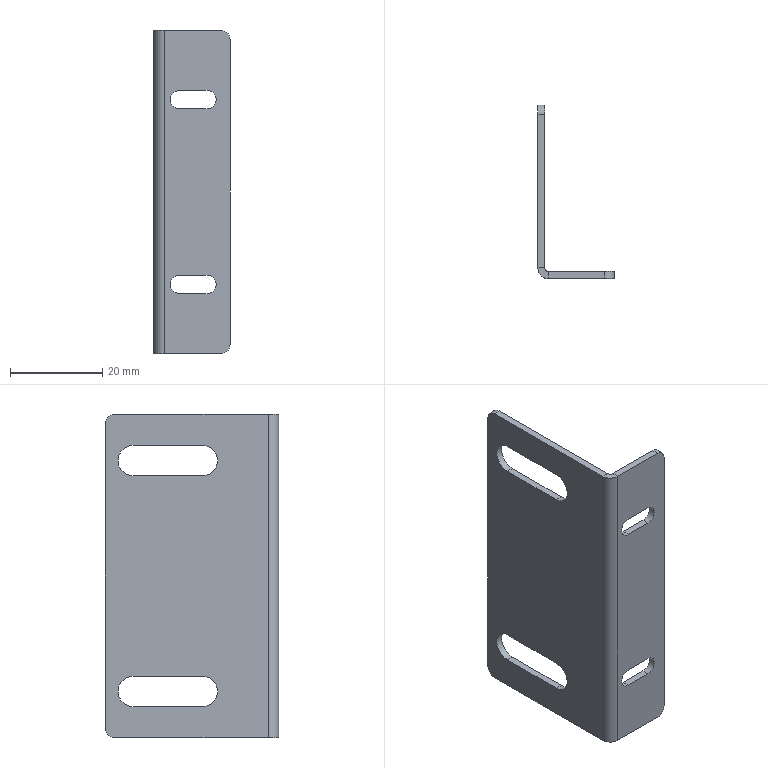Part | STEP file | 4R32456 | 1 solid | 34 faces | box 16.5 x 37.5 x 70 mm | volume 4931 mm3 | plane 20 | cylinder 14 | commonest cylinder face diameters 4 x8 6.6 x4 1.473 x1 4.473 x1